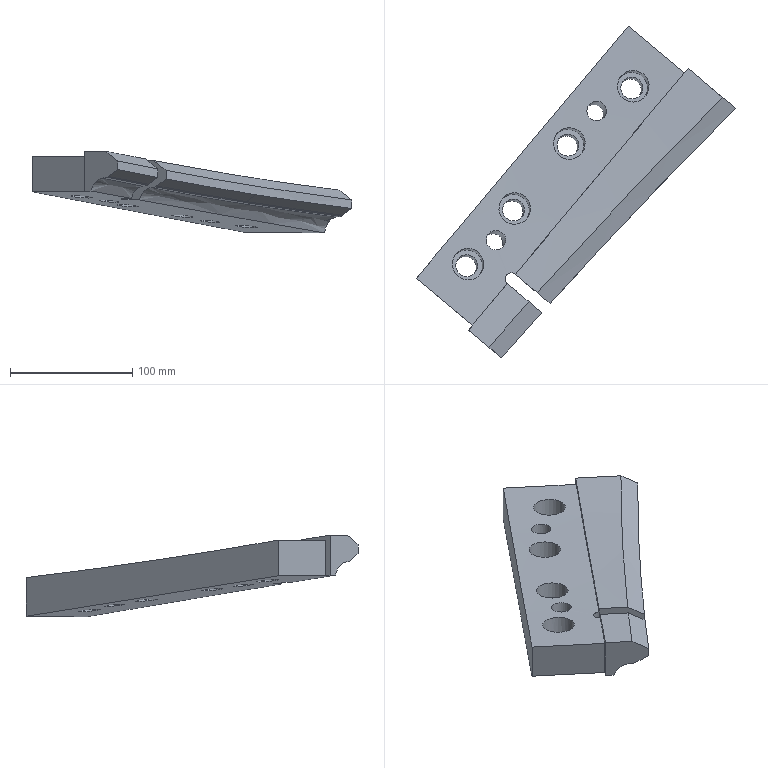Part | NX | features solid 2 | 1 solid | 43 faces | box 261.762 x 272.091 x 67.167 mm | volume 693128 mm3 | spline 18 | plane 14 | cylinder 11 | commonest cylinder face diameters 18 x4 26 x4 16 x2 10 x1